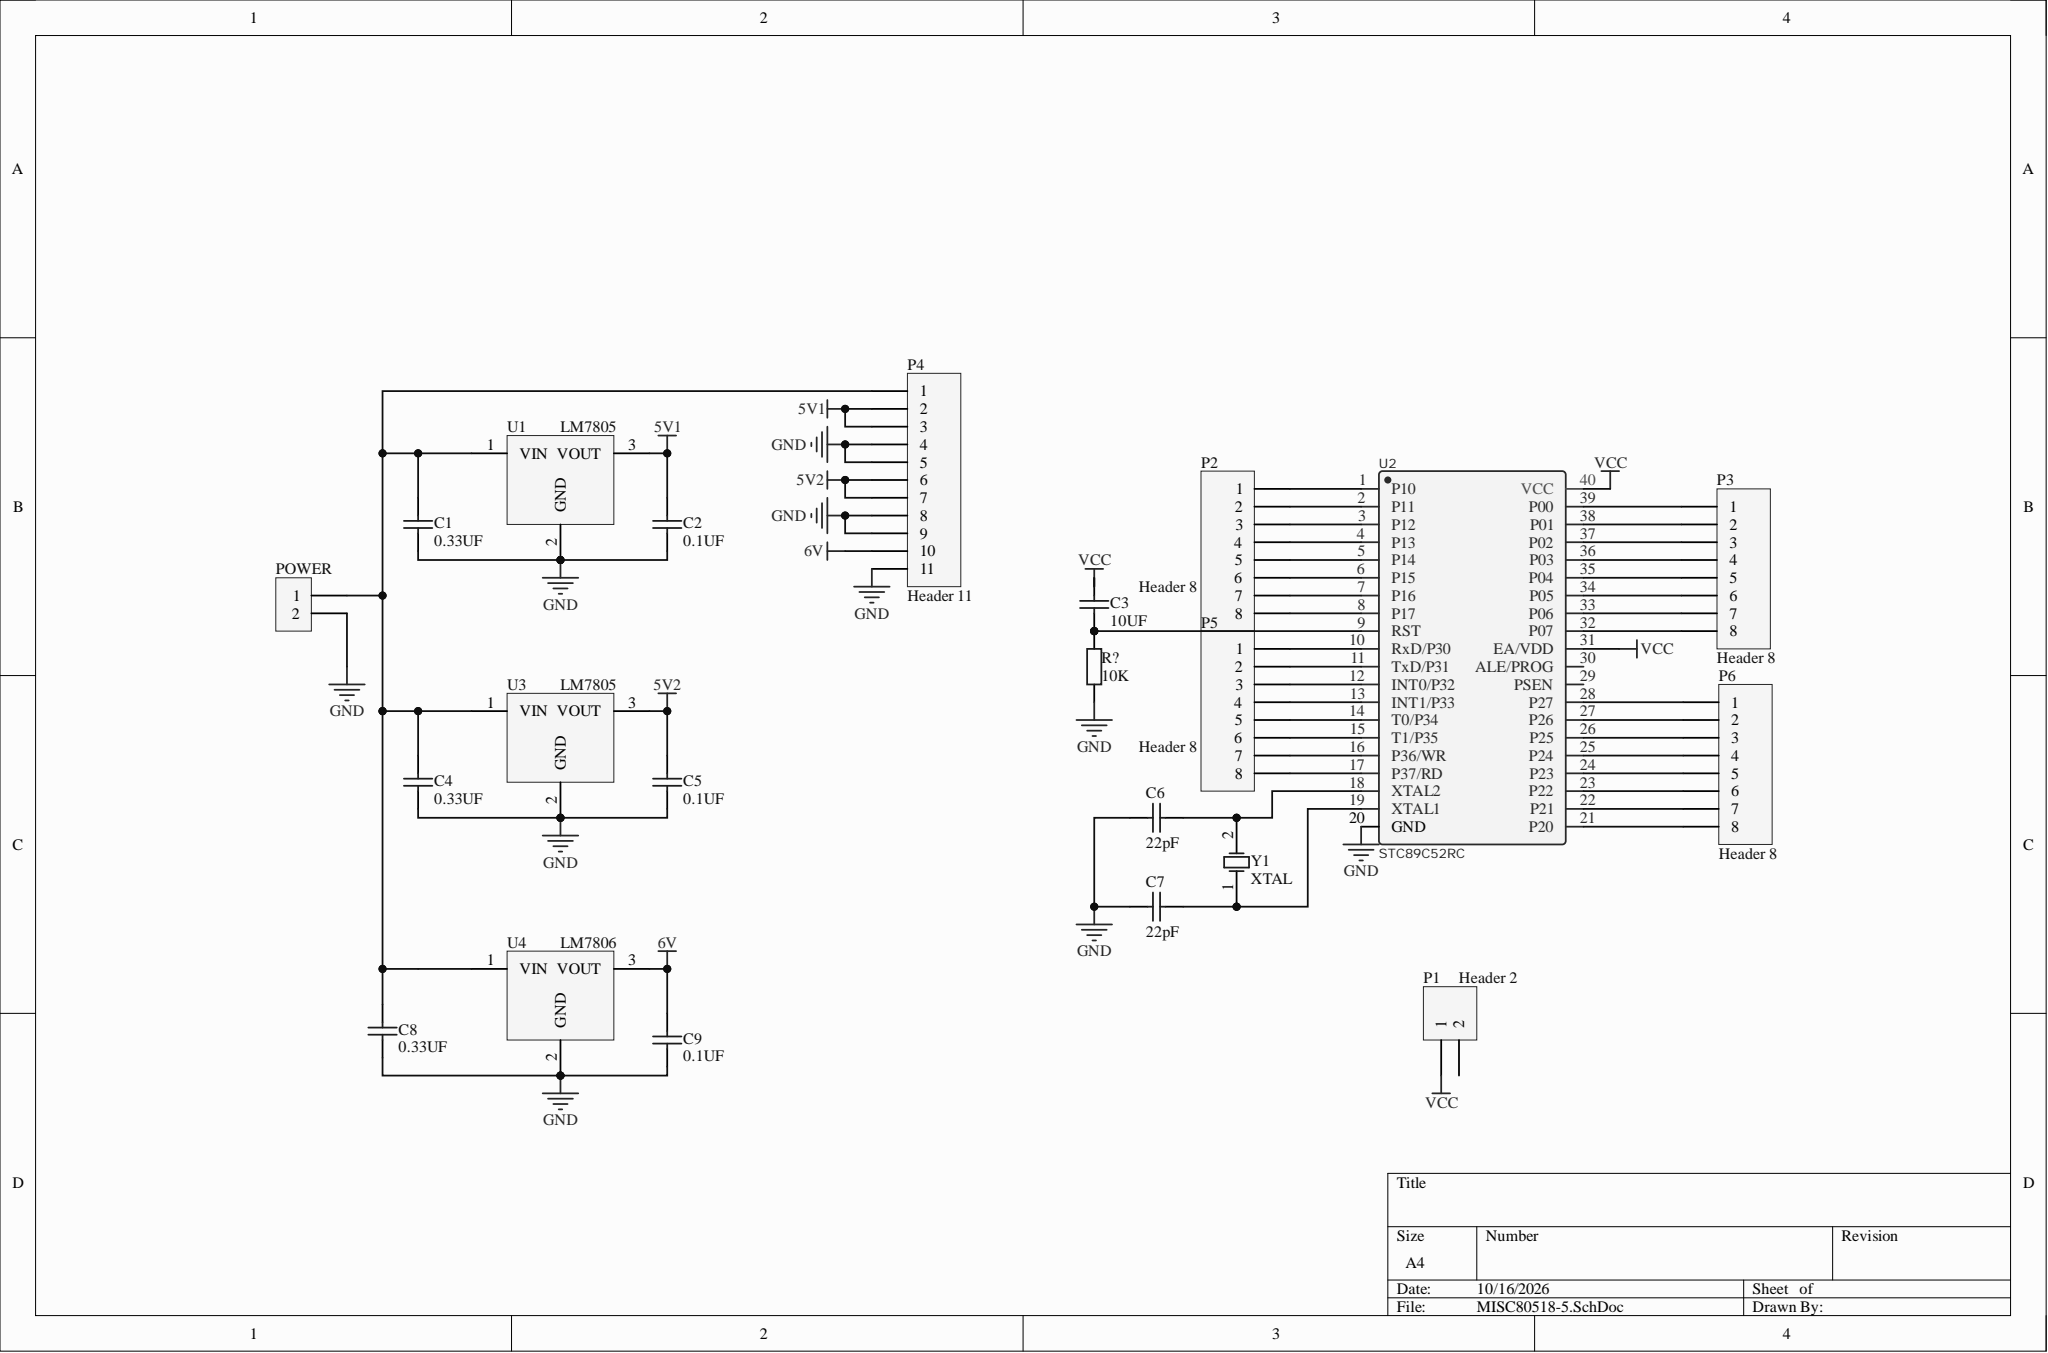Circuit board | Altium Designer | 22 parts | 41 nets
Bill of materials:
Comment,Description,Designator,Footprint,LibRef,Quantity
"0.33UF","Capacitor","C1, C4, C8","RAD-0.3","Cap","3"
"0.1UF","Capacitor","C2, C5, C9","RAD-0.3","Cap","3"
"10UF","Capacitor","C3","RAD-0.3","Cap","1"
"22pF","Capacitor","C6, C7","RAD-0.3","Cap","2"
"Header 2","Header, 2-Pin","P1","HDR1X2","Header 2","1"
"Header 8","Header, 8-Pin","P2, P3, P5, P6","HDR1X8","Header 8","4"
"Header 11","Header, 11-Pin","P4","HDR1X11","Header 11","1"
"Terminal block","","POWER","VH3.96-2A","VH2","1"
"10K","Resistor","R?","AXIAL-0.4","Res2","1"
"LM7805","","U1, U3","TO220A","LM7805","2"
"STC89C52RC","","U2","STC89C52RC","STC89C52RC","1"
"LM7806","","U4","TO220A","LM7805","1"
"XTAL","Crystal Oscillator","Y1","R38","XTAL","1"
Netlist (Protel format):
[
C1
RAD-0.3
0.33UF



]
[
C2
RAD-0.3
0.1UF



]
[
C3
RAD-0.3
10UF



]
[
C4
RAD-0.3
0.33UF



]
[
C5
RAD-0.3
0.1UF



]
[
C6
RAD-0.3
22pF



]
[
C7
RAD-0.3
22pF



]
[
C8
RAD-0.3
0.33UF



]
[
C9
RAD-0.3
0.1UF



]
[
P1
HDR1X2
Header 2



]
[
P2
HDR1X8
Header 8



]
[
P3
HDR1X8
Header 8



]
[
P4
HDR1X11
Header 11



]
[
P5
HDR1X8
Header 8



]
[
P6
HDR1X8
Header 8



]
[
POWER
VH3.96-2A
Terminal block



]
[
R?
AXIAL-0.4
10K



]
[
U1
TO220A
LM7805



]
[
U2
STC89C52RC
STC89C52RC



]
[
U3
TO220A
LM7805



]
[
U4
TO220A
LM7806



]
[
Y1
R38
XTAL



]
(
VCC
C3-1
P1-1
U2-31
U2-40
)
(
NetP6_8
P6-8
U2-21
)
(
NetP6_7
P6-7
U2-22
)
(
NetP6_6
P6-6
U2-23
)
(
NetP6_5
P6-5
U2-24
)
(
NetP6_4
P6-4
U2-25
)
(
NetP6_3
P6-3
U2-26
)
(
NetP6_2
P6-2
U2-27
)
(
NetP6_1
P6-1
U2-28
)
(
NetP5_8
P5-8
U2-17
)
(
NetP5_7
P5-7
U2-16
)
(
NetP5_6
P5-6
U2-15
)
(
NetP5_5
P5-5
U2-14
)
(
NetP5_4
P5-4
U2-13
)
(
NetP5_3
P5-3
U2-12
)
(
NetP5_2
P5-2
U2-11
)
(
NetP5_1
P5-1
U2-10
)
(
NetP3_8
P3-8
U2-32
)
(
NetP3_7
P3-7
U2-33
)
(
NetP3_6
P3-6
U2-34
)
(
NetP3_5
P3-5
U2-35
)
(
NetP3_4
P3-4
U2-36
)
(
NetP3_3
P3-3
U2-37
)
(
NetP3_2
P3-2
U2-38
)
(
NetP3_1
P3-1
U2-39
)
(
NetP2_8
P2-8
U2-8
)
(
NetP2_7
P2-7
U2-7
)
(
NetP2_6
P2-6
U2-6
)
(
NetP2_5
P2-5
U2-5
)
(
NetP2_4
P2-4
U2-4
)
(
NetP2_3
P2-3
U2-3
)
(
NetP2_2
P2-2
U2-2
)
(
NetP2_1
P2-1
U2-1
)
(
NetC7_1
C7-1
U2-19
Y1-1
)
(
NetC6_1
C6-1
U2-18
Y1-2
)
(
NetC3_2
C3-2
R?-2
U2-9
)
(
NetC1_1
C1-1
C4-1
C8-1
P4-1
POWER-1
U1-1
U3-1
U4-1
)
(
GND
C1-2
C2-2
C4-2
C5-2
C6-2
C7-2
C8-2
C9-2
P4-4
P4-5
P4-8
P4-9
P4-11
POWER-2
R?-1
U1-2
U2-20
U3-2
U4-2
)
(
6V
C9-1
P4-10
U4-3
)
(
5V2
C5-1
P4-6
P4-7
U3-3
)
(
5V1
C2-1
P4-2
P4-3
U1-3
)